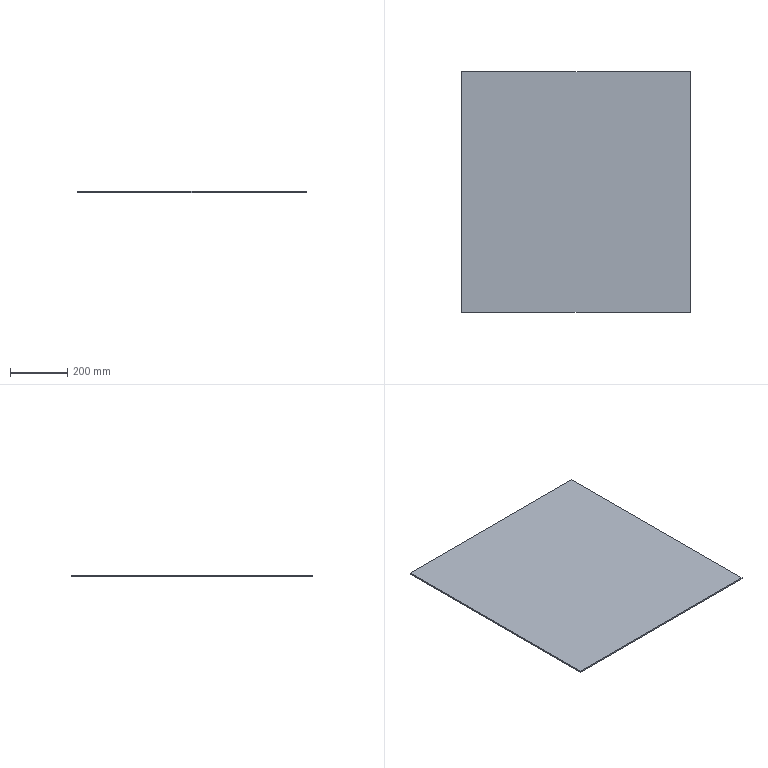Part | SolidWorks | features Extrusion 1, HoleWzd 1 | 1 solid | 6 faces | box 801 x 842 x 5 mm | volume 3372210 mm3 | plane 6
STEP:
#1=CARTESIAN_POINT('',(400.5,-421.,0.));
#2=VERTEX_POINT('',#1);
#3=CARTESIAN_POINT('',(400.5,421.,0.));
#4=VERTEX_POINT('',#3);
#5=CARTESIAN_POINT('',(400.5,421.,0.));
#6=DIRECTION('',(0.,1.,0.));
#7=VECTOR('',#6,1000.);
#8=LINE('',#5,#7);
#9=EDGE_CURVE('',#2,#4,#8,.T.);
#10=ORIENTED_EDGE('',*,*,#9,.T.);
#11=CARTESIAN_POINT('',(400.5,421.,5.));
#12=VERTEX_POINT('',#11);
#13=CARTESIAN_POINT('',(400.5,421.,5.));
#14=DIRECTION('',(0.,0.,-1.));
#15=VECTOR('',#14,1000.);
#16=LINE('',#13,#15);
#17=EDGE_CURVE('',#12,#4,#16,.T.);
#18=ORIENTED_EDGE('',*,*,#17,.F.);
#19=CARTESIAN_POINT('',(400.5,-421.,5.));
#20=VERTEX_POINT('',#19);
#21=CARTESIAN_POINT('',(400.5,421.,5.));
#22=DIRECTION('',(0.,1.,0.));
#23=VECTOR('',#22,1000.);
#24=LINE('',#21,#23);
#25=EDGE_CURVE('',#20,#12,#24,.T.);
#26=ORIENTED_EDGE('',*,*,#25,.F.);
#27=CARTESIAN_POINT('',(400.5,-421.,5.));
#28=DIRECTION('',(0.,0.,-1.));
#29=VECTOR('',#28,1000.);
#30=LINE('',#27,#29);
#31=EDGE_CURVE('',#20,#2,#30,.T.);
#32=ORIENTED_EDGE('',*,*,#31,.T.);
#33=EDGE_LOOP('',(#10,#18,#26,#32));
#34=FACE_OUTER_BOUND('',#33,.T.);
#35=CARTESIAN_POINT('',(400.5,421.,5.));
#36=DIRECTION('',(-1.,0.,0.));
#37=DIRECTION('',(0.,-1.,0.));
#38=AXIS2_PLACEMENT_3D('',#35,#36,#37);
#39=PLANE('',#38);
#40=ADVANCED_FACE('',(#34),#39,.F.);
#41=CARTESIAN_POINT('',(-400.5,421.,0.));
#42=VERTEX_POINT('',#41);
#43=CARTESIAN_POINT('',(-400.5,421.,0.));
#44=DIRECTION('',(-1.,0.,0.));
#45=VECTOR('',#44,1000.);
#46=LINE('',#43,#45);
#47=EDGE_CURVE('',#4,#42,#46,.T.);
#48=ORIENTED_EDGE('',*,*,#47,.T.);
#49=CARTESIAN_POINT('',(-400.5,421.,5.));
#50=VERTEX_POINT('',#49);
#51=CARTESIAN_POINT('',(-400.5,421.,5.));
#52=DIRECTION('',(0.,0.,-1.));
#53=VECTOR('',#52,1000.);
#54=LINE('',#51,#53);
#55=EDGE_CURVE('',#50,#42,#54,.T.);
#56=ORIENTED_EDGE('',*,*,#55,.F.);
#57=CARTESIAN_POINT('',(-400.5,421.,5.));
#58=DIRECTION('',(-1.,0.,0.));
#59=VECTOR('',#58,1000.);
#60=LINE('',#57,#59);
#61=EDGE_CURVE('',#12,#50,#60,.T.);
#62=ORIENTED_EDGE('',*,*,#61,.F.);
#63=ORIENTED_EDGE('',*,*,#17,.T.);
#64=EDGE_LOOP('',(#48,#56,#62,#63));
#65=FACE_OUTER_BOUND('',#64,.T.);
#66=CARTESIAN_POINT('',(-400.5,421.,5.));
#67=DIRECTION('',(0.,-1.,0.));
#68=DIRECTION('',(0.,0.,-1.));
#69=AXIS2_PLACEMENT_3D('',#66,#67,#68);
#70=PLANE('',#69);
#71=ADVANCED_FACE('',(#65),#70,.F.);
#72=CARTESIAN_POINT('',(-400.5,-421.,0.));
#73=VERTEX_POINT('',#72);
#74=CARTESIAN_POINT('',(-400.5,421.,0.));
#75=DIRECTION('',(0.,-1.,0.));
#76=VECTOR('',#75,1000.);
#77=LINE('',#74,#76);
#78=EDGE_CURVE('',#42,#73,#77,.T.);
#79=ORIENTED_EDGE('',*,*,#78,.T.);
#80=CARTESIAN_POINT('',(-400.5,-421.,5.));
#81=VERTEX_POINT('',#80);
#82=CARTESIAN_POINT('',(-400.5,-421.,5.));
#83=DIRECTION('',(0.,0.,-1.));
#84=VECTOR('',#83,1000.);
#85=LINE('',#82,#84);
#86=EDGE_CURVE('',#81,#73,#85,.T.);
#87=ORIENTED_EDGE('',*,*,#86,.F.);
#88=CARTESIAN_POINT('',(-400.5,421.,5.));
#89=DIRECTION('',(0.,-1.,0.));
#90=VECTOR('',#89,1000.);
#91=LINE('',#88,#90);
#92=EDGE_CURVE('',#50,#81,#91,.T.);
#93=ORIENTED_EDGE('',*,*,#92,.F.);
#94=ORIENTED_EDGE('',*,*,#55,.T.);
#95=EDGE_LOOP('',(#79,#87,#93,#94));
#96=FACE_OUTER_BOUND('',#95,.T.);
#97=CARTESIAN_POINT('',(-400.5,421.,5.));
#98=DIRECTION('',(1.,0.,0.));
#99=DIRECTION('',(0.,1.,0.));
#100=AXIS2_PLACEMENT_3D('',#97,#98,#99);
#101=PLANE('',#100);
#102=ADVANCED_FACE('',(#96),#101,.F.);
#103=CARTESIAN_POINT('',(-400.5,-421.,0.));
#104=DIRECTION('',(1.,0.,0.));
#105=VECTOR('',#104,1000.);
#106=LINE('',#103,#105);
#107=EDGE_CURVE('',#73,#2,#106,.T.);
#108=ORIENTED_EDGE('',*,*,#107,.T.);
#109=ORIENTED_EDGE('',*,*,#31,.F.);
#110=CARTESIAN_POINT('',(-400.5,-421.,5.));
#111=DIRECTION('',(1.,0.,0.));
#112=VECTOR('',#111,1000.);
#113=LINE('',#110,#112);
#114=EDGE_CURVE('',#81,#20,#113,.T.);
#115=ORIENTED_EDGE('',*,*,#114,.F.);
#116=ORIENTED_EDGE('',*,*,#86,.T.);
#117=EDGE_LOOP('',(#108,#109,#115,#116));
#118=FACE_OUTER_BOUND('',#117,.T.);
#119=CARTESIAN_POINT('',(-400.5,-421.,5.));
#120=DIRECTION('',(0.,1.,0.));
#121=DIRECTION('',(0.,0.,1.));
#122=AXIS2_PLACEMENT_3D('',#119,#120,#121);
#123=PLANE('',#122);
#124=ADVANCED_FACE('',(#118),#123,.F.);
#125=ORIENTED_EDGE('',*,*,#25,.T.);
#126=ORIENTED_EDGE('',*,*,#61,.T.);
#127=ORIENTED_EDGE('',*,*,#92,.T.);
#128=ORIENTED_EDGE('',*,*,#114,.T.);
#129=EDGE_LOOP('',(#125,#126,#127,#128));
#130=FACE_OUTER_BOUND('',#129,.T.);
#131=CARTESIAN_POINT('',(0.,0.,5.));
#132=DIRECTION('',(0.,0.,1.));
#133=DIRECTION('',(1.,0.,0.));
#134=AXIS2_PLACEMENT_3D('',#131,#132,#133);
#135=PLANE('',#134);
#136=ADVANCED_FACE('',(#130),#135,.T.);
#137=ORIENTED_EDGE('',*,*,#9,.F.);
#138=ORIENTED_EDGE('',*,*,#107,.F.);
#139=ORIENTED_EDGE('',*,*,#78,.F.);
#140=ORIENTED_EDGE('',*,*,#47,.F.);
#141=EDGE_LOOP('',(#137,#138,#139,#140));
#142=FACE_OUTER_BOUND('',#141,.T.);
#143=CARTESIAN_POINT('',(0.,0.,0.));
#144=DIRECTION('',(0.,0.,1.));
#145=DIRECTION('',(1.,0.,0.));
#146=AXIS2_PLACEMENT_3D('',#143,#144,#145);
#147=PLANE('',#146);
#148=ADVANCED_FACE('',(#142),#147,.F.);
#149=CLOSED_SHELL('',(#40,#71,#102,#124,#136,#148));
#150=MANIFOLD_SOLID_BREP('',#149);
#151=CARTESIAN_POINT('',(0.,0.,0.));
#152=DIRECTION('',(0.,0.,1.));
#153=DIRECTION('',(1.,0.,0.));
#154=AXIS2_PLACEMENT_3D('',#151,#152,#153);
#155=(LENGTH_UNIT()NAMED_UNIT(*)SI_UNIT(.MILLI.,.METRE.));
#156=UNCERTAINTY_MEASURE_WITH_UNIT(LENGTH_MEASURE(0.00001),#155,'','');
#157=(NAMED_UNIT(*)PLANE_ANGLE_UNIT()SI_UNIT($,.RADIAN.));
#158=(NAMED_UNIT(*)SI_UNIT($,.STERADIAN.)SOLID_ANGLE_UNIT());
#159=(GEOMETRIC_REPRESENTATION_CONTEXT(3)GLOBAL_UNCERTAINTY_ASSIGNED_CONTEXT((#156))GLOBAL_UNIT_ASSIGNED_CONTEXT((#155,#157,#158))REPRESENTATION_CONTEXT('',''));
#160=ADVANCED_BREP_SHAPE_REPRESENTATION('',(#150,#154),#159);